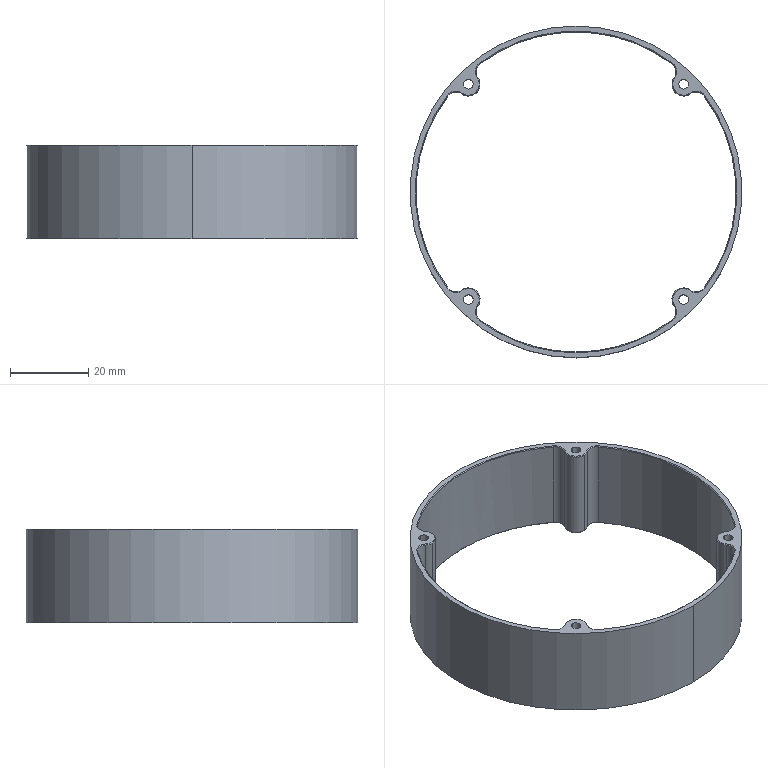NC program | NX | posted with a generic post | part box 85 x 85 x 24 mm
Lines 1 to 137 of 6793:
N10 G17 G21 G94 G90
(FLOOR_WALL_COPY , TOOL : D80)
N12 T19 M6
N14 G54
N16 G17 G0 G90 X-88.5 Y42.497 S6500 M3
N18 G43 Z30. H19
N20 Z8.
N22 G94 G1 Z5. F1500.
N24 X-82.5
N26 X82.5
N28 Y-10.5
N30 X-82.5
N32 X-88.5
N34 Z8.
N36 G0 Z30.
N38 Y42.497
N40 Z7.
N42 G1 Z4.
N44 X-82.5
N46 X82.5
N48 Y-10.5
N50 X-82.5
N52 X-88.5
N54 Z7.
N56 G0 Z30.
N58 Y42.497
N60 Z6.
N62 G1 Z3.
N64 X-82.5
N66 X82.5
N68 Y-10.5
N70 X-82.5
N72 X-88.5
N74 Z6.
N76 G0 Z30.
N78 Y42.497
N80 Z5.
N82 G1 Z2.
N84 X-82.5
N86 X82.5
N88 Y-10.5
N90 X-82.5
N92 X-88.5
N94 Z5.
N96 G0 Z30.
N98 Y42.497
N100 Z4.
N102 G1 Z1.
N104 X-82.5
N106 X82.5
N108 Y-10.5
N110 X-82.5
N112 X-88.5
N114 Z4.
N116 G0 Z30.
N118 Y42.497
N120 Z3.
N122 G1 Z0.
N124 X-82.5
N126 X82.5
N128 Y-10.5
N130 X-82.5
N132 X-88.5
N134 Z3.
N136 G0 Z30.
N138 M5
(DRILLING , TOOL : D6A45)
N140 T01 M6
N142 G54
N144 G17 G0 G90 X27.577 Y-27.577 S5000 M3
N146 G43 Z30. H1
N148 G94 G81 G98 Z-1.6 F350. R3.
N150 X-27.577
N152 Y27.577
N154 X27.577
N156 G80
N158 G0 X27.577 Y27.577 Z30.
(PLANAR_MILL_COPY_COPY_COPY_COPY_COPY_COPY_1_COPY , TOOL : D6A45)
N160 X0.866 Y-43.9 S9500
N162 Z0.5
N164 G1 Z-1. F1250.
N166 G3 X0. Y-43.4 R1.
N168 G2 X-43.4 Y0. R43.4
N170 X0. Y-43.4 R-43.4
N172 G3 X-0.866 Y-43.9 R1.
N174 G1 Z0.5
N176 G0 Z30.
(PLANAR_MILL_COPY_COPY_COPY_COPY_COPY_COPY_1_COPY_COPY , TOOL : D6A45)
N178 X-39.2 Y0.866
N180 Z1.5
N182 G1 Z-1.5 F800.
N184 G3 X-39.7 Y0. R1.
N186 X-31.75 Y-23.834 R39.7 F1250.
N188 X-30.089 Y-24.087 R1.2
N190 G2 X-24.087 Y-30.089 R4.3
N192 G3 X-23.834 Y-31.75 R1.2
N194 X23.834 Y-31.75 R39.7
N196 X24.087 Y-30.089 R1.2
N198 G2 X30.089 Y-24.087 R4.3
N200 G3 X31.75 Y-23.834 R1.2
N202 X31.75 Y23.834 R39.7
N204 X30.089 Y24.087 R1.2
N206 G2 X24.087 Y30.089 R4.3
N208 G3 X23.834 Y31.75 R1.2
N210 X-23.834 Y31.75 R39.7
N212 X-24.087 Y30.089 R1.2
N214 G2 X-30.089 Y24.087 R4.3
N216 G3 X-31.75 Y23.834 R1.2
N218 X-39.7 Y0. R39.7
N220 X-39.2 Y-0.866 R1.
N222 G1 Z1.5
N224 G0 Z30.
N226 M5
(DRILLING_COPY , TOOL : 2.5ZT)
N228 T02 M6
N230 G54
N232 G17 G0 G90 X27.577 Y-27.577 S2000 M3
N234 G43 Z30. H2
N236 G94 G83 G98 Z-26.251 F100. Q2. R3.
N238 X-27.577
N240 Y27.577
N242 X27.577
N244 G80
N246 G0 X27.577 Y27.577 Z30.
N248 M5